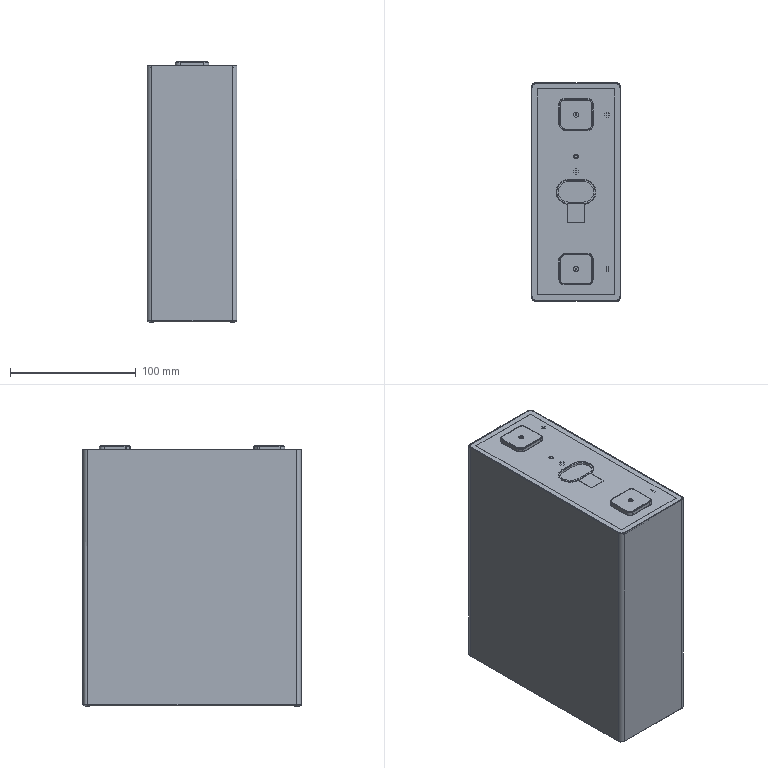Part | NX | features BREP 1 | 1 solid | 271 faces | box 71.65 x 173.93 x 207.23 mm | volume 2540512 mm3 | plane 174 | cylinder 87 | cone 6 | spline 4 | commonest cylinder face diameters 6 x20 2 x12 4 x12 4.22 x6 7.4 x6 8 x6